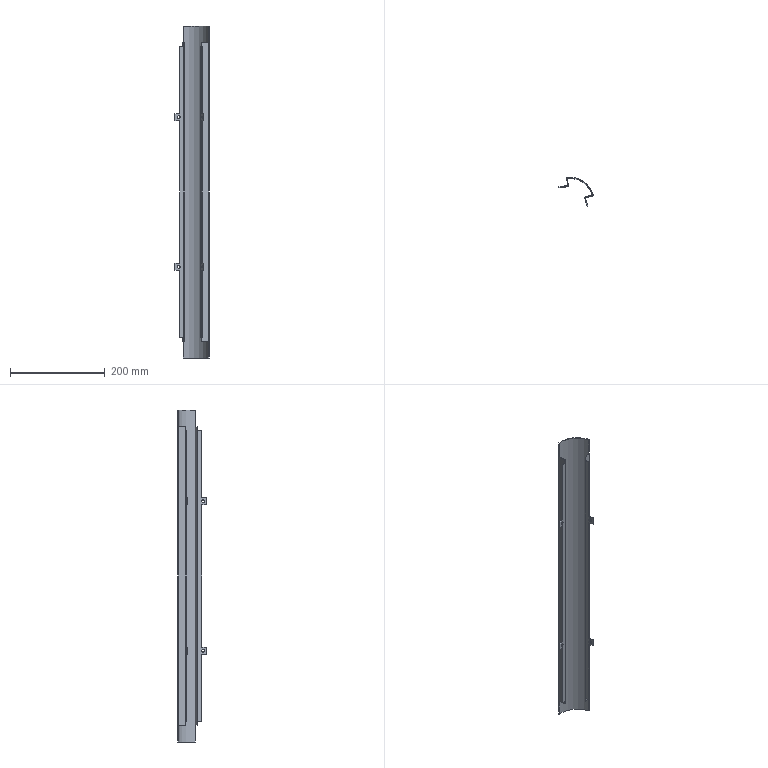Part | SolidWorks | features EdgeFlange 4, SMBaseFlange 3, ICE 2, FlatPattern 1, SheetMetal 1 | 1 solid | 66 faces | box 72.164 x 60.825 x 700 mm | volume 123678 mm3 | plane 52 | cylinder 14 | commonest cylinder face diameters 6 x8 3 x4 97 x1 100 x1